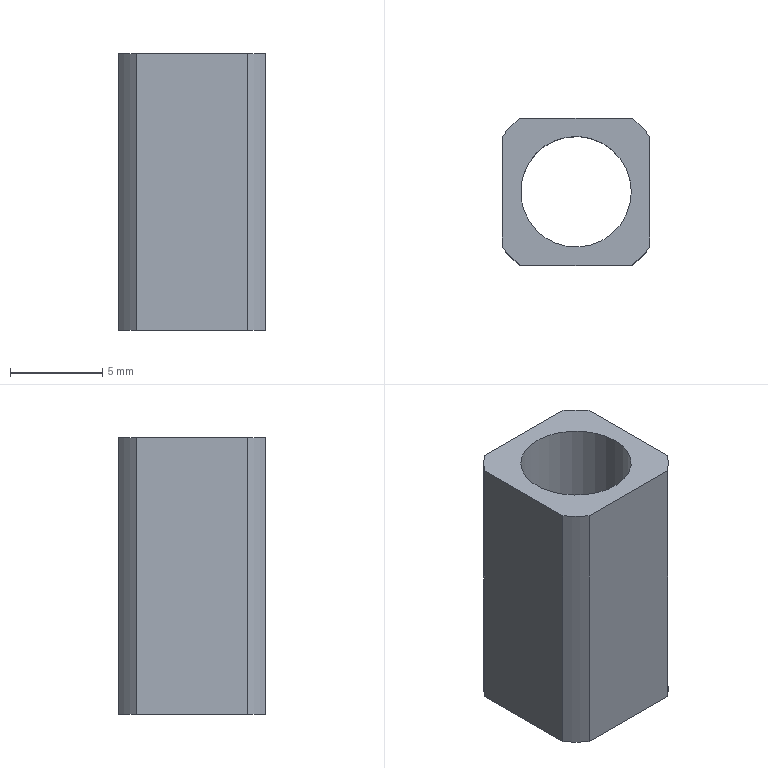CAM job | NX | 3-axis milling, drilling | part box 8 x 8 x 15 mm | stock box 16 x 16 x 25 mm
Tools:
number,name,description,diameter,corner_radius,flute_length,length,flutes
1,D8开粗,Milling Tool-5 Parameters,8.0,0.0,50.0,75.0,2
5,D6倒角刀,Milling Tool-5 Parameters,6.0,0.0,50.0,75.0,2
2,D8精光,Milling Tool-5 Parameters,8.0,0.0,50.0,75.0,2
3,D10点钻,Milling Tool-5 Parameters,10.0,0.0,50.0,75.0,2
4,5.1钻头,Milling Tool-5 Parameters,5.1,0.0,50.0,75.0,2
6,M6,Milling Tool-5 Parameters,6.0,0.0,50.0,75.0,2
7,D4,Milling Tool-5 Parameters,4.0,0.0,50.0,75.0,2
Operations:
program,operation,operation_type,tool,method,geometry_group,spindle_rpm,surface_speed,feed_per_tooth,feed_cut,feed_plunge,cut_length_mm,path_length_mm,cut_time_min,machine_time_min
G54,PLANAR_MILL,PlanarMilling,D8开粗,METHOD,WORKPIECE,2000.0,50.0,0.2,800.0,100.0,56.987,72.987,0.0712,0.0728
G54,ADAPTIVE_MILLING,CavityMilling,D8开粗,METHOD,WORKPIECE,3000.0,75.0,0.1667,1000.0,100.0,1136.193,1182.493,1.089,1.094
G54,DRILLING,Operation,D10点钻,METHOD,WORKPIECE,1200.0,37.0,0.0417,100.0,0.0,4.5,54.0,0.045,0.0499
G54,DRILLING_1,Operation,5.1钻头,METHOD,WORKPIECE,1600.0,25.0,0.0469,150.0,0.0,31.0,107.0,0.2067,0.2143
G54,DRILLING_COPY,Operation,D10点钻,METHOD,WORKPIECE,1600.0,25.0,0.0469,150.0,0.0,6.0,57.0,0.04,0.0451
G54,PLANAR_MILL_1,PlanarMilling,D4,METHOD,WORKPIECE,3000.0,43.0,0.0429,300.0,100.0,49.864,83.864,0.1662,0.1696
G54,DRILLING_1_COPY,Operation,M6,METHOD,WORKPIECE,300.0,5.0,0.0017,1.0,0.0,18.0,81.0,18.0,18.006
G54,PLANAR_MILL_3_COPY_1,PlanarMilling,D6倒角刀,METHOD,WORKPIECE,3000.0,56.0,0.1333,800.0,100.0,50.242,70.242,0.0628,0.0648
G54,PLANAR_MILL_COPY_COPY,PlanarMilling,D8精光,METHOD,WORKPIECE,3000.0,75.0,0.1,600.0,100.0,42.987,58.987,0.0716,0.0732
G54,PLANAR_MILL_1_COPY,PlanarMilling,D8精光,METHOD,WORKPIECE,3000.0,75.0,0.1,600.0,100.0,133.836,181.836,0.2231,0.2279